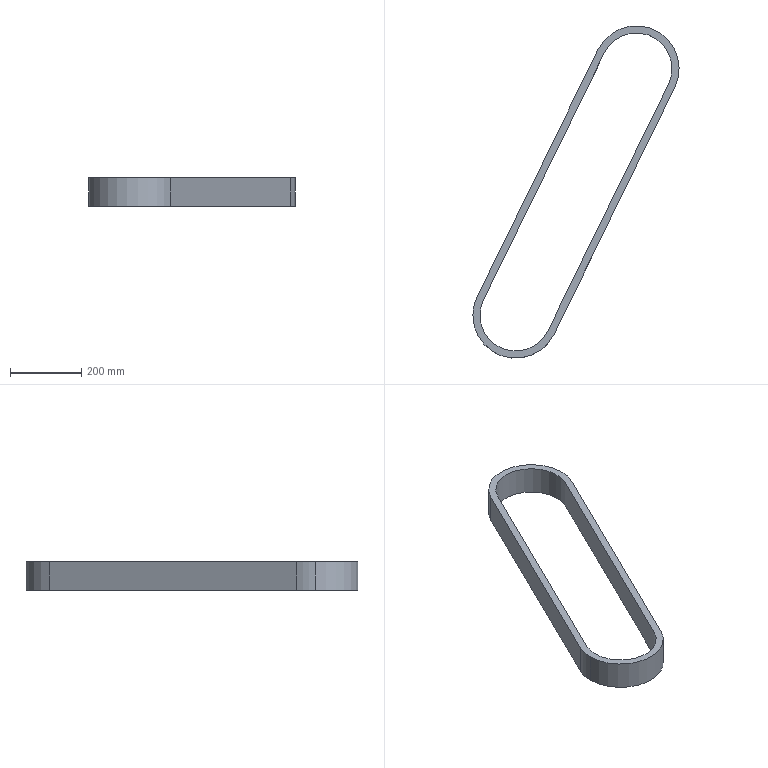Part | SolidWorks | features Extrusion 1 | 1 solid | 12 faces | box 578.858 x 932.782 x 80 mm | volume 3573726 mm3 | cylinder 6 | plane 6 | commonest cylinder face diameters 200 x3 240 x3
STEP:
#1=CARTESIAN_POINT('',(557.761,192.956,40.));
#2=VERTEX_POINT('',#1);
#3=CARTESIAN_POINT('',(547.591,149.017,40.));
#4=VERTEX_POINT('',#3);
#5=CARTESIAN_POINT('',(647.591,149.017,40.));
#6=DIRECTION('',(0.,0.,1.));
#7=DIRECTION('',(1.,0.,0.));
#8=AXIS2_PLACEMENT_3D('',#5,#6,#7);
#9=CIRCLE('',#8,100.);
#10=EDGE_CURVE('',#2,#4,#9,.T.);
#11=ORIENTED_EDGE('',*,*,#10,.T.);
#12=CARTESIAN_POINT('',(547.591,149.017,-40.));
#13=VERTEX_POINT('',#12);
#14=CARTESIAN_POINT('',(547.591,149.017,40.));
#15=DIRECTION('',(0.,0.,-1.));
#16=VECTOR('',#15,1000.);
#17=LINE('',#14,#16);
#18=EDGE_CURVE('',#4,#13,#17,.T.);
#19=ORIENTED_EDGE('',*,*,#18,.T.);
#20=CARTESIAN_POINT('',(557.761,192.956,-40.));
#21=VERTEX_POINT('',#20);
#22=CARTESIAN_POINT('',(647.591,149.017,-40.));
#23=DIRECTION('',(0.,0.,1.));
#24=DIRECTION('',(1.,0.,0.));
#25=AXIS2_PLACEMENT_3D('',#22,#23,#24);
#26=CIRCLE('',#25,100.);
#27=EDGE_CURVE('',#21,#13,#26,.T.);
#28=ORIENTED_EDGE('',*,*,#27,.F.);
#29=CARTESIAN_POINT('',(557.761,192.956,40.));
#30=DIRECTION('',(0.,0.,-1.));
#31=VECTOR('',#30,1000.);
#32=LINE('',#29,#31);
#33=EDGE_CURVE('',#2,#21,#32,.T.);
#34=ORIENTED_EDGE('',*,*,#33,.F.);
#35=EDGE_LOOP('',(#11,#19,#28,#34));
#36=FACE_OUTER_BOUND('',#35,.T.);
#37=CARTESIAN_POINT('',(647.591,149.017,40.));
#38=DIRECTION('',(0.,0.,-1.));
#39=DIRECTION('',(-1.,0.,0.));
#40=AXIS2_PLACEMENT_3D('',#37,#38,#39);
#41=CYLINDRICAL_SURFACE('',#40,100.);
#42=ADVANCED_FACE('',(#36),#41,.F.);
#43=CARTESIAN_POINT('',(527.591,149.017,40.));
#44=VERTEX_POINT('',#43);
#45=CARTESIAN_POINT('',(755.387,96.292,40.));
#46=VERTEX_POINT('',#45);
#47=CARTESIAN_POINT('',(647.591,149.017,40.));
#48=DIRECTION('',(0.,0.,1.));
#49=DIRECTION('',(1.,0.,0.));
#50=AXIS2_PLACEMENT_3D('',#47,#48,#49);
#51=CIRCLE('',#50,120.);
#52=EDGE_CURVE('',#44,#46,#51,.T.);
#53=ORIENTED_EDGE('',*,*,#52,.F.);
#54=CARTESIAN_POINT('',(527.591,149.017,-40.));
#55=VERTEX_POINT('',#54);
#56=CARTESIAN_POINT('',(527.591,149.017,40.));
#57=DIRECTION('',(0.,0.,-1.));
#58=VECTOR('',#57,1000.);
#59=LINE('',#56,#58);
#60=EDGE_CURVE('',#44,#55,#59,.T.);
#61=ORIENTED_EDGE('',*,*,#60,.T.);
#62=CARTESIAN_POINT('',(755.387,96.292,-40.));
#63=VERTEX_POINT('',#62);
#64=CARTESIAN_POINT('',(647.591,149.017,-40.));
#65=DIRECTION('',(0.,0.,1.));
#66=DIRECTION('',(1.,0.,0.));
#67=AXIS2_PLACEMENT_3D('',#64,#65,#66);
#68=CIRCLE('',#67,120.);
#69=EDGE_CURVE('',#55,#63,#68,.T.);
#70=ORIENTED_EDGE('',*,*,#69,.T.);
#71=CARTESIAN_POINT('',(755.387,96.292,40.));
#72=DIRECTION('',(0.,0.,-1.));
#73=VECTOR('',#72,1000.);
#74=LINE('',#71,#73);
#75=EDGE_CURVE('',#46,#63,#74,.T.);
#76=ORIENTED_EDGE('',*,*,#75,.F.);
#77=EDGE_LOOP('',(#53,#61,#70,#76));
#78=FACE_OUTER_BOUND('',#77,.T.);
#79=CARTESIAN_POINT('',(647.591,149.017,40.));
#80=DIRECTION('',(0.,0.,-1.));
#81=DIRECTION('',(-1.,0.,0.));
#82=AXIS2_PLACEMENT_3D('',#79,#80,#81);
#83=CYLINDRICAL_SURFACE('',#82,120.);
#84=ADVANCED_FACE('',(#78),#83,.T.);
#85=CARTESIAN_POINT('',(1094.245,789.074,40.));
#86=VERTEX_POINT('',#85);
#87=CARTESIAN_POINT('',(878.653,894.525,40.));
#88=VERTEX_POINT('',#87);
#89=CARTESIAN_POINT('',(986.449,841.799,40.));
#90=DIRECTION('',(0.,0.,1.));
#91=DIRECTION('',(1.,0.,0.));
#92=AXIS2_PLACEMENT_3D('',#89,#90,#91);
#93=CIRCLE('',#92,120.);
#94=EDGE_CURVE('',#86,#88,#93,.T.);
#95=ORIENTED_EDGE('',*,*,#94,.T.);
#96=CARTESIAN_POINT('',(539.795,201.743,40.));
#97=VERTEX_POINT('',#96);
#98=CARTESIAN_POINT('',(878.653,894.525,40.));
#99=DIRECTION('',(-0.4394,-0.8983,0.));
#100=VECTOR('',#99,1000.);
#101=LINE('',#98,#100);
#102=EDGE_CURVE('',#88,#97,#101,.T.);
#103=ORIENTED_EDGE('',*,*,#102,.T.);
#104=CARTESIAN_POINT('',(647.591,149.017,40.));
#105=DIRECTION('',(0.,0.,1.));
#106=DIRECTION('',(1.,0.,0.));
#107=AXIS2_PLACEMENT_3D('',#104,#105,#106);
#108=CIRCLE('',#107,120.);
#109=EDGE_CURVE('',#97,#44,#108,.T.);
#110=ORIENTED_EDGE('',*,*,#109,.T.);
#111=ORIENTED_EDGE('',*,*,#52,.T.);
#112=CARTESIAN_POINT('',(1094.245,789.074,40.));
#113=DIRECTION('',(0.4394,0.8983,0.));
#114=VECTOR('',#113,1000.);
#115=LINE('',#112,#114);
#116=EDGE_CURVE('',#46,#86,#115,.T.);
#117=ORIENTED_EDGE('',*,*,#116,.T.);
#118=EDGE_LOOP('',(#95,#103,#110,#111,#117));
#119=FACE_OUTER_BOUND('',#118,.T.);
#120=CARTESIAN_POINT('',(896.619,885.738,40.));
#121=VERTEX_POINT('',#120);
#122=CARTESIAN_POINT('',(896.619,885.738,40.));
#123=DIRECTION('',(-0.4394,-0.8983,0.));
#124=VECTOR('',#123,1000.);
#125=LINE('',#122,#124);
#126=EDGE_CURVE('',#121,#2,#125,.T.);
#127=ORIENTED_EDGE('',*,*,#126,.F.);
#128=CARTESIAN_POINT('',(1076.279,797.861,40.));
#129=VERTEX_POINT('',#128);
#130=CARTESIAN_POINT('',(986.449,841.799,40.));
#131=DIRECTION('',(0.,0.,1.));
#132=DIRECTION('',(1.,0.,0.));
#133=AXIS2_PLACEMENT_3D('',#130,#131,#132);
#134=CIRCLE('',#133,100.);
#135=EDGE_CURVE('',#129,#121,#134,.T.);
#136=ORIENTED_EDGE('',*,*,#135,.F.);
#137=CARTESIAN_POINT('',(737.421,105.079,40.));
#138=VERTEX_POINT('',#137);
#139=CARTESIAN_POINT('',(1076.279,797.861,40.));
#140=DIRECTION('',(0.4394,0.8983,0.));
#141=VECTOR('',#140,1000.);
#142=LINE('',#139,#141);
#143=EDGE_CURVE('',#138,#129,#142,.T.);
#144=ORIENTED_EDGE('',*,*,#143,.F.);
#145=CARTESIAN_POINT('',(647.591,149.017,40.));
#146=DIRECTION('',(0.,0.,1.));
#147=DIRECTION('',(1.,0.,0.));
#148=AXIS2_PLACEMENT_3D('',#145,#146,#147);
#149=CIRCLE('',#148,100.);
#150=EDGE_CURVE('',#4,#138,#149,.T.);
#151=ORIENTED_EDGE('',*,*,#150,.F.);
#152=ORIENTED_EDGE('',*,*,#10,.F.);
#153=EDGE_LOOP('',(#127,#136,#144,#151,#152));
#154=FACE_BOUND('',#153,.T.);
#155=CARTESIAN_POINT('',(986.449,841.799,40.));
#156=DIRECTION('',(0.,0.,1.));
#157=DIRECTION('',(1.,0.,0.));
#158=AXIS2_PLACEMENT_3D('',#155,#156,#157);
#159=PLANE('',#158);
#160=ADVANCED_FACE('',(#119,#154),#159,.T.);
#161=CARTESIAN_POINT('',(1094.245,789.074,-40.));
#162=VERTEX_POINT('',#161);
#163=CARTESIAN_POINT('',(878.653,894.525,-40.));
#164=VERTEX_POINT('',#163);
#165=CARTESIAN_POINT('',(986.449,841.799,-40.));
#166=DIRECTION('',(0.,0.,1.));
#167=DIRECTION('',(1.,0.,0.));
#168=AXIS2_PLACEMENT_3D('',#165,#166,#167);
#169=CIRCLE('',#168,120.);
#170=EDGE_CURVE('',#162,#164,#169,.T.);
#171=ORIENTED_EDGE('',*,*,#170,.F.);
#172=CARTESIAN_POINT('',(1094.245,789.074,-40.));
#173=DIRECTION('',(0.4394,0.8983,0.));
#174=VECTOR('',#173,1000.);
#175=LINE('',#172,#174);
#176=EDGE_CURVE('',#63,#162,#175,.T.);
#177=ORIENTED_EDGE('',*,*,#176,.F.);
#178=ORIENTED_EDGE('',*,*,#69,.F.);
#179=CARTESIAN_POINT('',(539.795,201.743,-40.));
#180=VERTEX_POINT('',#179);
#181=CARTESIAN_POINT('',(647.591,149.017,-40.));
#182=DIRECTION('',(0.,0.,1.));
#183=DIRECTION('',(1.,0.,0.));
#184=AXIS2_PLACEMENT_3D('',#181,#182,#183);
#185=CIRCLE('',#184,120.);
#186=EDGE_CURVE('',#180,#55,#185,.T.);
#187=ORIENTED_EDGE('',*,*,#186,.F.);
#188=CARTESIAN_POINT('',(878.653,894.525,-40.));
#189=DIRECTION('',(-0.4394,-0.8983,0.));
#190=VECTOR('',#189,1000.);
#191=LINE('',#188,#190);
#192=EDGE_CURVE('',#164,#180,#191,.T.);
#193=ORIENTED_EDGE('',*,*,#192,.F.);
#194=EDGE_LOOP('',(#171,#177,#178,#187,#193));
#195=FACE_OUTER_BOUND('',#194,.T.);
#196=CARTESIAN_POINT('',(1076.279,797.861,-40.));
#197=VERTEX_POINT('',#196);
#198=CARTESIAN_POINT('',(896.619,885.738,-40.));
#199=VERTEX_POINT('',#198);
#200=CARTESIAN_POINT('',(986.449,841.799,-40.));
#201=DIRECTION('',(0.,0.,1.));
#202=DIRECTION('',(1.,0.,0.));
#203=AXIS2_PLACEMENT_3D('',#200,#201,#202);
#204=CIRCLE('',#203,100.);
#205=EDGE_CURVE('',#197,#199,#204,.T.);
#206=ORIENTED_EDGE('',*,*,#205,.T.);
#207=CARTESIAN_POINT('',(896.619,885.738,-40.));
#208=DIRECTION('',(-0.4394,-0.8983,0.));
#209=VECTOR('',#208,1000.);
#210=LINE('',#207,#209);
#211=EDGE_CURVE('',#199,#21,#210,.T.);
#212=ORIENTED_EDGE('',*,*,#211,.T.);
#213=ORIENTED_EDGE('',*,*,#27,.T.);
#214=CARTESIAN_POINT('',(737.421,105.079,-40.));
#215=VERTEX_POINT('',#214);
#216=CARTESIAN_POINT('',(647.591,149.017,-40.));
#217=DIRECTION('',(0.,0.,1.));
#218=DIRECTION('',(1.,0.,0.));
#219=AXIS2_PLACEMENT_3D('',#216,#217,#218);
#220=CIRCLE('',#219,100.);
#221=EDGE_CURVE('',#13,#215,#220,.T.);
#222=ORIENTED_EDGE('',*,*,#221,.T.);
#223=CARTESIAN_POINT('',(1076.279,797.861,-40.));
#224=DIRECTION('',(0.4394,0.8983,0.));
#225=VECTOR('',#224,1000.);
#226=LINE('',#223,#225);
#227=EDGE_CURVE('',#215,#197,#226,.T.);
#228=ORIENTED_EDGE('',*,*,#227,.T.);
#229=EDGE_LOOP('',(#206,#212,#213,#222,#228));
#230=FACE_BOUND('',#229,.T.);
#231=CARTESIAN_POINT('',(986.449,841.799,-40.));
#232=DIRECTION('',(0.,0.,1.));
#233=DIRECTION('',(1.,0.,0.));
#234=AXIS2_PLACEMENT_3D('',#231,#232,#233);
#235=PLANE('',#234);
#236=ADVANCED_FACE('',(#195,#230),#235,.F.);
#237=ORIENTED_EDGE('',*,*,#170,.T.);
#238=CARTESIAN_POINT('',(878.653,894.525,40.));
#239=DIRECTION('',(0.,0.,-1.));
#240=VECTOR('',#239,1000.);
#241=LINE('',#238,#240);
#242=EDGE_CURVE('',#88,#164,#241,.T.);
#243=ORIENTED_EDGE('',*,*,#242,.F.);
#244=ORIENTED_EDGE('',*,*,#94,.F.);
#245=CARTESIAN_POINT('',(1094.245,789.074,40.));
#246=DIRECTION('',(0.,0.,-1.));
#247=VECTOR('',#246,1000.);
#248=LINE('',#245,#247);
#249=EDGE_CURVE('',#86,#162,#248,.T.);
#250=ORIENTED_EDGE('',*,*,#249,.T.);
#251=EDGE_LOOP('',(#237,#243,#244,#250));
#252=FACE_OUTER_BOUND('',#251,.T.);
#253=CARTESIAN_POINT('',(986.449,841.799,40.));
#254=DIRECTION('',(0.,0.,-1.));
#255=DIRECTION('',(-1.,0.,0.));
#256=AXIS2_PLACEMENT_3D('',#253,#254,#255);
#257=CYLINDRICAL_SURFACE('',#256,120.);
#258=ADVANCED_FACE('',(#252),#257,.T.);
#259=ORIENTED_EDGE('',*,*,#192,.T.);
#260=CARTESIAN_POINT('',(539.795,201.743,40.));
#261=DIRECTION('',(0.,0.,-1.));
#262=VECTOR('',#261,1000.);
#263=LINE('',#260,#262);
#264=EDGE_CURVE('',#97,#180,#263,.T.);
#265=ORIENTED_EDGE('',*,*,#264,.F.);
#266=ORIENTED_EDGE('',*,*,#102,.F.);
#267=ORIENTED_EDGE('',*,*,#242,.T.);
#268=EDGE_LOOP('',(#259,#265,#266,#267));
#269=FACE_OUTER_BOUND('',#268,.T.);
#270=CARTESIAN_POINT('',(878.653,894.525,40.));
#271=DIRECTION('',(0.8983,-0.4394,0.));
#272=DIRECTION('',(0.4394,0.8983,0.));
#273=AXIS2_PLACEMENT_3D('',#270,#271,#272);
#274=PLANE('',#273);
#275=ADVANCED_FACE('',(#269),#274,.F.);
#276=ORIENTED_EDGE('',*,*,#60,.F.);
#277=ORIENTED_EDGE('',*,*,#109,.F.);
#278=ORIENTED_EDGE('',*,*,#264,.T.);
#279=ORIENTED_EDGE('',*,*,#186,.T.);
#280=EDGE_LOOP('',(#276,#277,#278,#279));
#281=FACE_OUTER_BOUND('',#280,.T.);
#282=CARTESIAN_POINT('',(647.591,149.017,40.));
#283=DIRECTION('',(0.,0.,-1.));
#284=DIRECTION('',(-1.,0.,0.));
#285=AXIS2_PLACEMENT_3D('',#282,#283,#284);
#286=CYLINDRICAL_SURFACE('',#285,120.);
#287=ADVANCED_FACE('',(#281),#286,.T.);
#288=ORIENTED_EDGE('',*,*,#176,.T.);
#289=ORIENTED_EDGE('',*,*,#249,.F.);
#290=ORIENTED_EDGE('',*,*,#116,.F.);
#291=ORIENTED_EDGE('',*,*,#75,.T.);
#292=EDGE_LOOP('',(#288,#289,#290,#291));
#293=FACE_OUTER_BOUND('',#292,.T.);
#294=CARTESIAN_POINT('',(1094.245,789.074,40.));
#295=DIRECTION('',(-0.8983,0.4394,0.));
#296=DIRECTION('',(-0.4394,-0.8983,0.));
#297=AXIS2_PLACEMENT_3D('',#294,#295,#296);
#298=PLANE('',#297);
#299=ADVANCED_FACE('',(#293),#298,.F.);
#300=ORIENTED_EDGE('',*,*,#205,.F.);
#301=CARTESIAN_POINT('',(1076.279,797.861,40.));
#302=DIRECTION('',(0.,0.,-1.));
#303=VECTOR('',#302,1000.);
#304=LINE('',#301,#303);
#305=EDGE_CURVE('',#129,#197,#304,.T.);
#306=ORIENTED_EDGE('',*,*,#305,.F.);
#307=ORIENTED_EDGE('',*,*,#135,.T.);
#308=CARTESIAN_POINT('',(896.619,885.738,40.));
#309=DIRECTION('',(0.,0.,-1.));
#310=VECTOR('',#309,1000.);
#311=LINE('',#308,#310);
#312=EDGE_CURVE('',#121,#199,#311,.T.);
#313=ORIENTED_EDGE('',*,*,#312,.T.);
#314=EDGE_LOOP('',(#300,#306,#307,#313));
#315=FACE_OUTER_BOUND('',#314,.T.);
#316=CARTESIAN_POINT('',(986.449,841.799,40.));
#317=DIRECTION('',(0.,0.,-1.));
#318=DIRECTION('',(-1.,0.,0.));
#319=AXIS2_PLACEMENT_3D('',#316,#317,#318);
#320=CYLINDRICAL_SURFACE('',#319,100.);
#321=ADVANCED_FACE('',(#315),#320,.F.);
#322=ORIENTED_EDGE('',*,*,#211,.F.);
#323=ORIENTED_EDGE('',*,*,#312,.F.);
#324=ORIENTED_EDGE('',*,*,#126,.T.);
#325=ORIENTED_EDGE('',*,*,#33,.T.);
#326=EDGE_LOOP('',(#322,#323,#324,#325));
#327=FACE_OUTER_BOUND('',#326,.T.);
#328=CARTESIAN_POINT('',(896.619,885.738,40.));
#329=DIRECTION('',(0.8983,-0.4394,0.));
#330=DIRECTION('',(0.4394,0.8983,0.));
#331=AXIS2_PLACEMENT_3D('',#328,#329,#330);
#332=PLANE('',#331);
#333=ADVANCED_FACE('',(#327),#332,.T.);
#334=ORIENTED_EDGE('',*,*,#18,.F.);
#335=ORIENTED_EDGE('',*,*,#150,.T.);
#336=CARTESIAN_POINT('',(737.421,105.079,40.));
#337=DIRECTION('',(0.,0.,-1.));
#338=VECTOR('',#337,1000.);
#339=LINE('',#336,#338);
#340=EDGE_CURVE('',#138,#215,#339,.T.);
#341=ORIENTED_EDGE('',*,*,#340,.T.);
#342=ORIENTED_EDGE('',*,*,#221,.F.);
#343=EDGE_LOOP('',(#334,#335,#341,#342));
#344=FACE_OUTER_BOUND('',#343,.T.);
#345=CARTESIAN_POINT('',(647.591,149.017,40.));
#346=DIRECTION('',(0.,0.,-1.));
#347=DIRECTION('',(-1.,0.,0.));
#348=AXIS2_PLACEMENT_3D('',#345,#346,#347);
#349=CYLINDRICAL_SURFACE('',#348,100.);
#350=ADVANCED_FACE('',(#344),#349,.F.);
#351=ORIENTED_EDGE('',*,*,#227,.F.);
#352=ORIENTED_EDGE('',*,*,#340,.F.);
#353=ORIENTED_EDGE('',*,*,#143,.T.);
#354=ORIENTED_EDGE('',*,*,#305,.T.);
#355=EDGE_LOOP('',(#351,#352,#353,#354));
#356=FACE_OUTER_BOUND('',#355,.T.);
#357=CARTESIAN_POINT('',(1076.279,797.861,40.));
#358=DIRECTION('',(-0.8983,0.4394,0.));
#359=DIRECTION('',(-0.4394,-0.8983,0.));
#360=AXIS2_PLACEMENT_3D('',#357,#358,#359);
#361=PLANE('',#360);
#362=ADVANCED_FACE('',(#356),#361,.T.);
#363=CLOSED_SHELL('',(#42,#84,#160,#236,#258,#275,#287,#299,#321,#333,#350,#362));
#364=MANIFOLD_SOLID_BREP('',#363);
#365=CARTESIAN_POINT('',(0.,0.,0.));
#366=DIRECTION('',(0.,0.,1.));
#367=DIRECTION('',(1.,0.,0.));
#368=AXIS2_PLACEMENT_3D('',#365,#366,#367);
#369=(LENGTH_UNIT()NAMED_UNIT(*)SI_UNIT(.MILLI.,.METRE.));
#370=UNCERTAINTY_MEASURE_WITH_UNIT(LENGTH_MEASURE(0.00001),#369,'','');
#371=(NAMED_UNIT(*)PLANE_ANGLE_UNIT()SI_UNIT($,.RADIAN.));
#372=(NAMED_UNIT(*)SI_UNIT($,.STERADIAN.)SOLID_ANGLE_UNIT());
#373=(GEOMETRIC_REPRESENTATION_CONTEXT(3)GLOBAL_UNCERTAINTY_ASSIGNED_CONTEXT((#370))GLOBAL_UNIT_ASSIGNED_CONTEXT((#369,#371,#372))REPRESENTATION_CONTEXT('',''));
#374=ADVANCED_BREP_SHAPE_REPRESENTATION('',(#364,#368),#373);